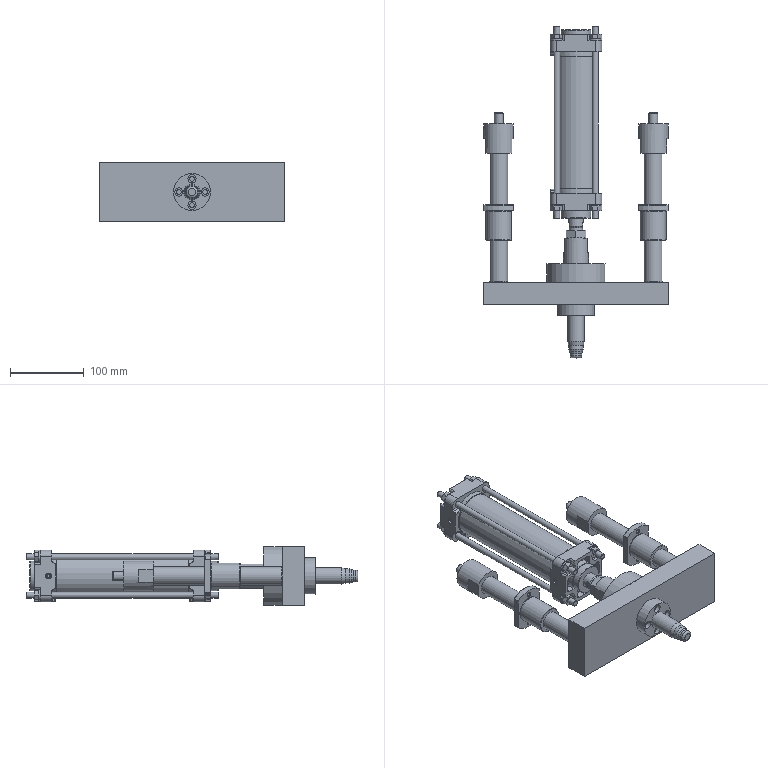Part | NX | features Hydraulic support1 2, Hydraulic support2 2, Hydraulic2.1_50 2, Hydraulic2.2_50 2, Hydraulic2.3_M18X1.5 2, Part2 2, bushing 2, clamp shaft 2, clamp stopper 2, mandrel expand 2 | 13 solids | 517 faces | box 250 x 451 x 80 mm | volume 1627599 mm3 | plane 296 | cylinder 177 | cone 38 | spline 4 | torus 2 | commonest cylinder face diameters 4 x34 6 x16 5 x12 8 x12 20 x11 18 x10